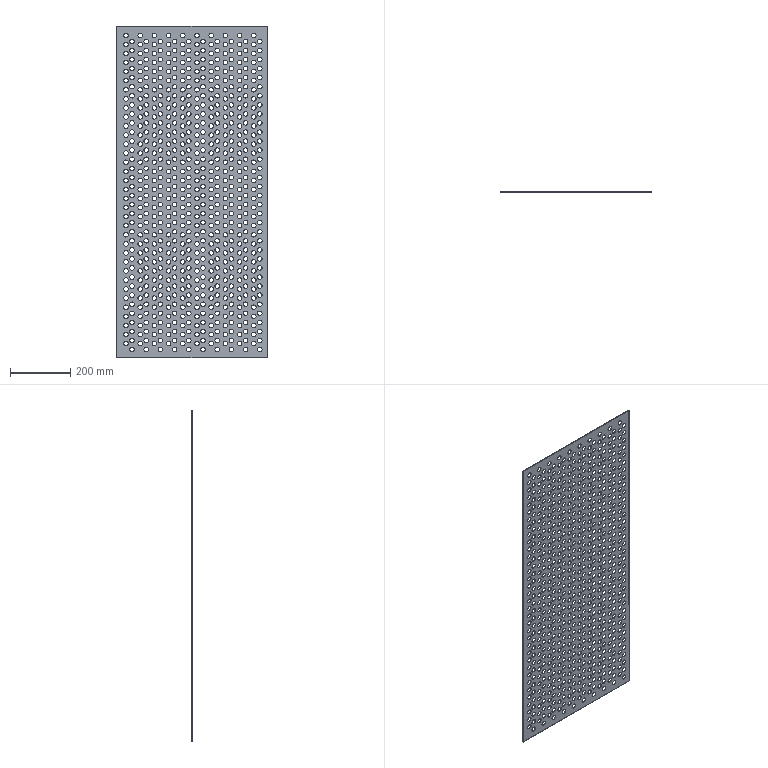Part | SolidWorks | features LPattern 2, FlatPattern 1, ICE 1, SMBaseFlange 1, SheetMetal 1 | 1 solid | 1406 faces | box 497 x 1.2 x 1097 mm | volume 505811 mm3 | cylinder 1400 | plane 6 | commonest cylinder face diameters 15 x1400